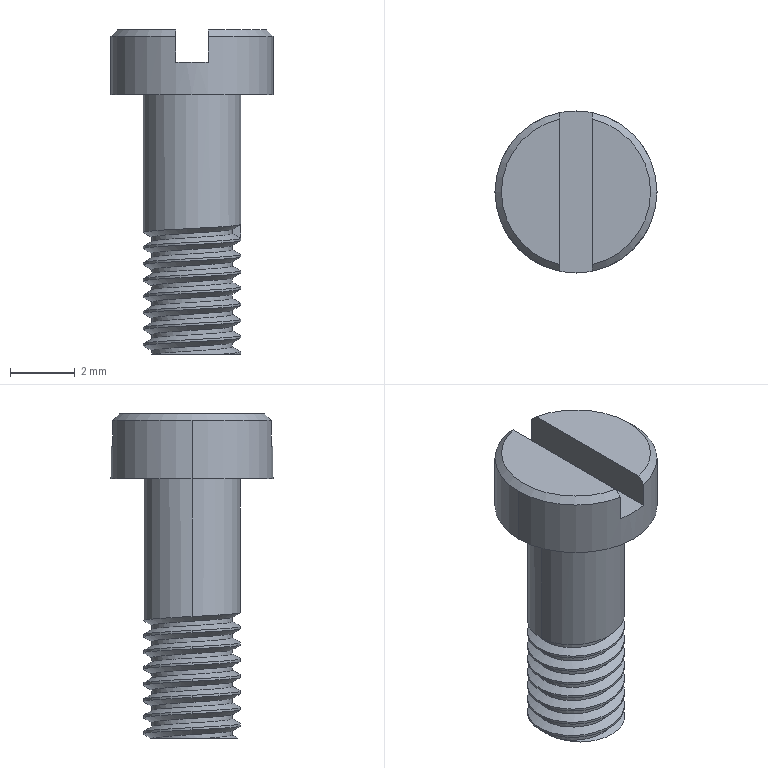Part | SolidWorks | features ICE 2, Extrusion 1, Helix 1, RevCut 1, SweepCut 1 | 1 solid | 32 faces | box 5 x 5 x 10 mm | volume 85.863 mm3 | cylinder 19 | plane 8 | spline 3 | cone 2 | commonest cylinder face diameters 3 x17 5 x2